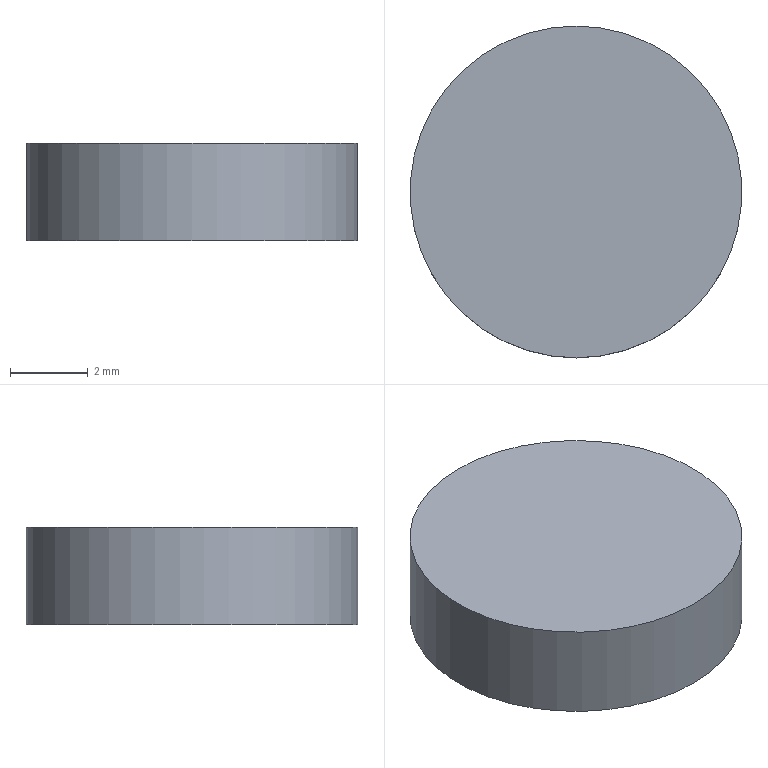Part | STEP file | lll_id406_x_t | 1 solid | 3 faces | box 8.55 x 8.55 x 2.5 mm | volume 143.536 mm3 | plane 2 | cylinder 1 | commonest cylinder face diameters 8.55 x1
STEP:
#1=CARTESIAN_POINT('',(3690.5,-55.225,-17.5));
#2=VERTEX_POINT('',#1);
#3=CARTESIAN_POINT('',(3690.5,-59.5,-17.5));
#4=DIRECTION('',(-0.000000008,0.,1.));
#5=DIRECTION('',(0.,1.,0.));
#6=AXIS2_PLACEMENT_3D('',#3,#4,#5);
#7=CIRCLE('',#6,4.275);
#8=EDGE_CURVE('',#2,#2,#7,.T.);
#9=ORIENTED_EDGE('',*,*,#8,.F.);
#10=EDGE_LOOP('',(#9));
#11=FACE_OUTER_BOUND('',#10,.T.);
#12=CARTESIAN_POINT('',(3690.5,-59.5,-17.5));
#13=DIRECTION('',(0.000000008,0.,-1.));
#14=DIRECTION('',(0.,1.,0.));
#15=AXIS2_PLACEMENT_3D('',#12,#13,#14);
#16=PLANE('',#15);
#17=ADVANCED_FACE('',(#11),#16,.T.);
#18=CARTESIAN_POINT('',(3690.5,-55.225,-15.));
#19=VERTEX_POINT('',#18);
#20=CARTESIAN_POINT('',(3690.5,-59.5,-15.));
#21=DIRECTION('',(-0.000000008,0.,1.));
#22=DIRECTION('',(0.,1.,0.));
#23=AXIS2_PLACEMENT_3D('',#20,#21,#22);
#24=CIRCLE('',#23,4.275);
#25=EDGE_CURVE('',#19,#19,#24,.T.);
#26=ORIENTED_EDGE('',*,*,#25,.T.);
#27=EDGE_LOOP('',(#26));
#28=FACE_OUTER_BOUND('',#27,.T.);
#29=CARTESIAN_POINT('',(3690.5,-59.5,-15.));
#30=DIRECTION('',(-0.000000008,0.,1.));
#31=DIRECTION('',(0.,-1.,0.));
#32=AXIS2_PLACEMENT_3D('',#29,#30,#31);
#33=PLANE('',#32);
#34=ADVANCED_FACE('',(#28),#33,.T.);
#35=ORIENTED_EDGE('',*,*,#8,.T.);
#36=EDGE_LOOP('',(#35));
#37=FACE_BOUND('',#36,.T.);
#38=ORIENTED_EDGE('',*,*,#25,.F.);
#39=EDGE_LOOP('',(#38));
#40=FACE_BOUND('',#39,.T.);
#41=CARTESIAN_POINT('',(3690.5,-59.5,-15.));
#42=DIRECTION('',(0.000000008,0.,-1.));
#43=DIRECTION('',(0.,1.,0.));
#44=AXIS2_PLACEMENT_3D('',#41,#42,#43);
#45=CYLINDRICAL_SURFACE('',#44,4.275);
#46=ADVANCED_FACE('',(#37,#40),#45,.T.);
#47=CLOSED_SHELL('',(#17,#34,#46));
#48=MANIFOLD_SOLID_BREP('',#47);
#49=(LENGTH_UNIT()NAMED_UNIT(*)SI_UNIT(.MILLI.,.METRE.));
#50=UNCERTAINTY_MEASURE_WITH_UNIT(LENGTH_MEASURE(0.00002),#49,'','');
#51=(NAMED_UNIT(*)PLANE_ANGLE_UNIT()SI_UNIT($,.RADIAN.));
#52=PLANE_ANGLE_MEASURE_WITH_UNIT(PLANE_ANGLE_MEASURE(0.01745),#51);
#53=DIMENSIONAL_EXPONENTS(0.,0.,0.,0.,0.,0.,0.);
#54=(CONVERSION_BASED_UNIT('DEGREE',#52)NAMED_UNIT(#53)PLANE_ANGLE_UNIT());
#55=(NAMED_UNIT(*)SI_UNIT($,.STERADIAN.)SOLID_ANGLE_UNIT());
#56=(GEOMETRIC_REPRESENTATION_CONTEXT(3)GLOBAL_UNCERTAINTY_ASSIGNED_CONTEXT((#50))GLOBAL_UNIT_ASSIGNED_CONTEXT((#49,#54,#55))REPRESENTATION_CONTEXT('',''));
#57=ADVANCED_BREP_SHAPE_REPRESENTATION('',(#48),#56);